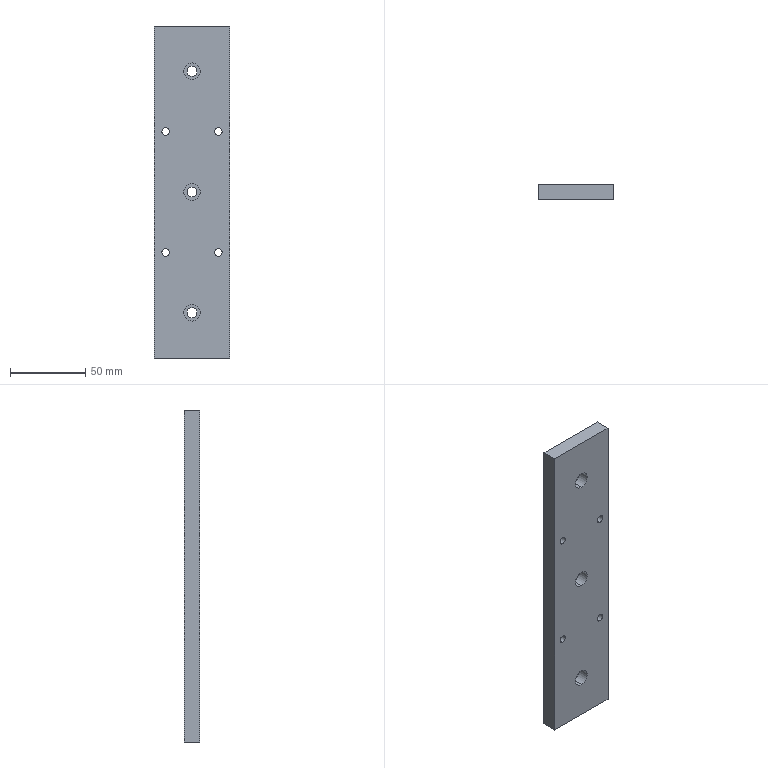Part | SolidWorks | features HoleWzd 2, Extrusion 1 | 1 solid | 29 faces | box 50 x 10 x 220 mm | volume 106947 mm3 | cylinder 20 | plane 9 | commonest cylinder face diameters 5 x8 6.6 x6 11 x6
STEP:
#1=CARTESIAN_POINT('',(-17.5,0.,-37.5));
#2=VERTEX_POINT('',#1);
#3=CARTESIAN_POINT('',(-17.5,0.,-42.5));
#4=VERTEX_POINT('',#3);
#5=CARTESIAN_POINT('',(-17.5,0.,-40.));
#6=DIRECTION('',(0.,-1.,0.));
#7=DIRECTION('',(0.,0.,-1.));
#8=AXIS2_PLACEMENT_3D('',#5,#6,#7);
#9=CIRCLE('',#8,2.5);
#10=EDGE_CURVE('',#2,#4,#9,.T.);
#11=ORIENTED_EDGE('',*,*,#10,.T.);
#12=CARTESIAN_POINT('',(-17.5,10.,-42.5));
#13=VERTEX_POINT('',#12);
#14=CARTESIAN_POINT('',(-17.5,10.,-42.5));
#15=DIRECTION('',(0.,1.,0.));
#16=VECTOR('',#15,1000.);
#17=LINE('',#14,#16);
#18=EDGE_CURVE('',#4,#13,#17,.T.);
#19=ORIENTED_EDGE('',*,*,#18,.T.);
#20=CARTESIAN_POINT('',(-17.5,10.,-37.5));
#21=VERTEX_POINT('',#20);
#22=CARTESIAN_POINT('',(-17.5,10.,-40.));
#23=DIRECTION('',(0.,1.,0.));
#24=DIRECTION('',(0.,0.,1.));
#25=AXIS2_PLACEMENT_3D('',#22,#23,#24);
#26=CIRCLE('',#25,2.5);
#27=EDGE_CURVE('',#13,#21,#26,.T.);
#28=ORIENTED_EDGE('',*,*,#27,.T.);
#29=CARTESIAN_POINT('',(-17.5,10.,-37.5));
#30=DIRECTION('',(0.,1.,0.));
#31=VECTOR('',#30,1000.);
#32=LINE('',#29,#31);
#33=EDGE_CURVE('',#2,#21,#32,.T.);
#34=ORIENTED_EDGE('',*,*,#33,.F.);
#35=EDGE_LOOP('',(#11,#19,#28,#34));
#36=FACE_OUTER_BOUND('',#35,.T.);
#37=CARTESIAN_POINT('',(-17.5,10.,-40.));
#38=DIRECTION('',(0.,1.,0.));
#39=DIRECTION('',(0.,0.,1.));
#40=AXIS2_PLACEMENT_3D('',#37,#38,#39);
#41=CYLINDRICAL_SURFACE('',#40,2.5);
#42=ADVANCED_FACE('',(#36),#41,.F.);
#43=CARTESIAN_POINT('',(-17.5,0.,42.5));
#44=VERTEX_POINT('',#43);
#45=CARTESIAN_POINT('',(-17.5,0.,37.5));
#46=VERTEX_POINT('',#45);
#47=CARTESIAN_POINT('',(-17.5,0.,40.));
#48=DIRECTION('',(0.,-1.,0.));
#49=DIRECTION('',(0.,0.,-1.));
#50=AXIS2_PLACEMENT_3D('',#47,#48,#49);
#51=CIRCLE('',#50,2.5);
#52=EDGE_CURVE('',#44,#46,#51,.T.);
#53=ORIENTED_EDGE('',*,*,#52,.T.);
#54=CARTESIAN_POINT('',(-17.5,10.,37.5));
#55=VERTEX_POINT('',#54);
#56=CARTESIAN_POINT('',(-17.5,10.,37.5));
#57=DIRECTION('',(0.,1.,0.));
#58=VECTOR('',#57,1000.);
#59=LINE('',#56,#58);
#60=EDGE_CURVE('',#46,#55,#59,.T.);
#61=ORIENTED_EDGE('',*,*,#60,.T.);
#62=CARTESIAN_POINT('',(-17.5,10.,42.5));
#63=VERTEX_POINT('',#62);
#64=CARTESIAN_POINT('',(-17.5,10.,40.));
#65=DIRECTION('',(0.,1.,0.));
#66=DIRECTION('',(0.,0.,1.));
#67=AXIS2_PLACEMENT_3D('',#64,#65,#66);
#68=CIRCLE('',#67,2.5);
#69=EDGE_CURVE('',#55,#63,#68,.T.);
#70=ORIENTED_EDGE('',*,*,#69,.T.);
#71=CARTESIAN_POINT('',(-17.5,10.,42.5));
#72=DIRECTION('',(0.,1.,0.));
#73=VECTOR('',#72,1000.);
#74=LINE('',#71,#73);
#75=EDGE_CURVE('',#44,#63,#74,.T.);
#76=ORIENTED_EDGE('',*,*,#75,.F.);
#77=EDGE_LOOP('',(#53,#61,#70,#76));
#78=FACE_OUTER_BOUND('',#77,.T.);
#79=CARTESIAN_POINT('',(-17.5,10.,40.));
#80=DIRECTION('',(0.,1.,0.));
#81=DIRECTION('',(0.,0.,1.));
#82=AXIS2_PLACEMENT_3D('',#79,#80,#81);
#83=CYLINDRICAL_SURFACE('',#82,2.5);
#84=ADVANCED_FACE('',(#78),#83,.F.);
#85=CARTESIAN_POINT('',(17.5,0.,-37.5));
#86=VERTEX_POINT('',#85);
#87=CARTESIAN_POINT('',(17.5,0.,-42.5));
#88=VERTEX_POINT('',#87);
#89=CARTESIAN_POINT('',(17.5,0.,-40.));
#90=DIRECTION('',(0.,-1.,0.));
#91=DIRECTION('',(0.,0.,-1.));
#92=AXIS2_PLACEMENT_3D('',#89,#90,#91);
#93=CIRCLE('',#92,2.5);
#94=EDGE_CURVE('',#86,#88,#93,.T.);
#95=ORIENTED_EDGE('',*,*,#94,.T.);
#96=CARTESIAN_POINT('',(17.5,10.,-42.5));
#97=VERTEX_POINT('',#96);
#98=CARTESIAN_POINT('',(17.5,10.,-42.5));
#99=DIRECTION('',(0.,1.,0.));
#100=VECTOR('',#99,1000.);
#101=LINE('',#98,#100);
#102=EDGE_CURVE('',#88,#97,#101,.T.);
#103=ORIENTED_EDGE('',*,*,#102,.T.);
#104=CARTESIAN_POINT('',(17.5,10.,-37.5));
#105=VERTEX_POINT('',#104);
#106=CARTESIAN_POINT('',(17.5,10.,-40.));
#107=DIRECTION('',(0.,1.,0.));
#108=DIRECTION('',(0.,0.,1.));
#109=AXIS2_PLACEMENT_3D('',#106,#107,#108);
#110=CIRCLE('',#109,2.5);
#111=EDGE_CURVE('',#97,#105,#110,.T.);
#112=ORIENTED_EDGE('',*,*,#111,.T.);
#113=CARTESIAN_POINT('',(17.5,10.,-37.5));
#114=DIRECTION('',(0.,1.,0.));
#115=VECTOR('',#114,1000.);
#116=LINE('',#113,#115);
#117=EDGE_CURVE('',#86,#105,#116,.T.);
#118=ORIENTED_EDGE('',*,*,#117,.F.);
#119=EDGE_LOOP('',(#95,#103,#112,#118));
#120=FACE_OUTER_BOUND('',#119,.T.);
#121=CARTESIAN_POINT('',(17.5,10.,-40.));
#122=DIRECTION('',(0.,1.,0.));
#123=DIRECTION('',(0.,0.,1.));
#124=AXIS2_PLACEMENT_3D('',#121,#122,#123);
#125=CYLINDRICAL_SURFACE('',#124,2.5);
#126=ADVANCED_FACE('',(#120),#125,.F.);
#127=CARTESIAN_POINT('',(17.5,0.,42.5));
#128=VERTEX_POINT('',#127);
#129=CARTESIAN_POINT('',(17.5,0.,37.5));
#130=VERTEX_POINT('',#129);
#131=CARTESIAN_POINT('',(17.5,0.,40.));
#132=DIRECTION('',(0.,-1.,0.));
#133=DIRECTION('',(0.,0.,-1.));
#134=AXIS2_PLACEMENT_3D('',#131,#132,#133);
#135=CIRCLE('',#134,2.5);
#136=EDGE_CURVE('',#128,#130,#135,.T.);
#137=ORIENTED_EDGE('',*,*,#136,.T.);
#138=CARTESIAN_POINT('',(17.5,10.,37.5));
#139=VERTEX_POINT('',#138);
#140=CARTESIAN_POINT('',(17.5,10.,37.5));
#141=DIRECTION('',(0.,1.,0.));
#142=VECTOR('',#141,1000.);
#143=LINE('',#140,#142);
#144=EDGE_CURVE('',#130,#139,#143,.T.);
#145=ORIENTED_EDGE('',*,*,#144,.T.);
#146=CARTESIAN_POINT('',(17.5,10.,42.5));
#147=VERTEX_POINT('',#146);
#148=CARTESIAN_POINT('',(17.5,10.,40.));
#149=DIRECTION('',(0.,1.,0.));
#150=DIRECTION('',(0.,0.,1.));
#151=AXIS2_PLACEMENT_3D('',#148,#149,#150);
#152=CIRCLE('',#151,2.5);
#153=EDGE_CURVE('',#139,#147,#152,.T.);
#154=ORIENTED_EDGE('',*,*,#153,.T.);
#155=CARTESIAN_POINT('',(17.5,10.,42.5));
#156=DIRECTION('',(0.,1.,0.));
#157=VECTOR('',#156,1000.);
#158=LINE('',#155,#157);
#159=EDGE_CURVE('',#128,#147,#158,.T.);
#160=ORIENTED_EDGE('',*,*,#159,.F.);
#161=EDGE_LOOP('',(#137,#145,#154,#160));
#162=FACE_OUTER_BOUND('',#161,.T.);
#163=CARTESIAN_POINT('',(17.5,10.,40.));
#164=DIRECTION('',(0.,1.,0.));
#165=DIRECTION('',(0.,0.,1.));
#166=AXIS2_PLACEMENT_3D('',#163,#164,#165);
#167=CYLINDRICAL_SURFACE('',#166,2.5);
#168=ADVANCED_FACE('',(#162),#167,.F.);
#169=CARTESIAN_POINT('',(0.,6.8,85.5));
#170=VERTEX_POINT('',#169);
#171=CARTESIAN_POINT('',(0.,6.8,74.5));
#172=VERTEX_POINT('',#171);
#173=CARTESIAN_POINT('',(0.,6.8,80.));
#174=DIRECTION('',(0.,-1.,0.));
#175=DIRECTION('',(0.,0.,-1.));
#176=AXIS2_PLACEMENT_3D('',#173,#174,#175);
#177=CIRCLE('',#176,5.5);
#178=EDGE_CURVE('',#170,#172,#177,.T.);
#179=ORIENTED_EDGE('',*,*,#178,.F.);
#180=CARTESIAN_POINT('',(0.,0.,85.5));
#181=VERTEX_POINT('',#180);
#182=CARTESIAN_POINT('',(0.,0.,85.5));
#183=DIRECTION('',(0.,-1.,0.));
#184=VECTOR('',#183,1000.);
#185=LINE('',#182,#184);
#186=EDGE_CURVE('',#170,#181,#185,.T.);
#187=ORIENTED_EDGE('',*,*,#186,.T.);
#188=CARTESIAN_POINT('',(0.,0.,74.5));
#189=VERTEX_POINT('',#188);
#190=CARTESIAN_POINT('',(0.,0.,80.));
#191=DIRECTION('',(0.,-1.,0.));
#192=DIRECTION('',(0.,0.,-1.));
#193=AXIS2_PLACEMENT_3D('',#190,#191,#192);
#194=CIRCLE('',#193,5.5);
#195=EDGE_CURVE('',#181,#189,#194,.T.);
#196=ORIENTED_EDGE('',*,*,#195,.T.);
#197=CARTESIAN_POINT('',(0.,0.,74.5));
#198=DIRECTION('',(0.,-1.,0.));
#199=VECTOR('',#198,1000.);
#200=LINE('',#197,#199);
#201=EDGE_CURVE('',#172,#189,#200,.T.);
#202=ORIENTED_EDGE('',*,*,#201,.F.);
#203=EDGE_LOOP('',(#179,#187,#196,#202));
#204=FACE_OUTER_BOUND('',#203,.T.);
#205=CARTESIAN_POINT('',(0.,0.,80.));
#206=DIRECTION('',(0.,-1.,0.));
#207=DIRECTION('',(0.,0.,-1.));
#208=AXIS2_PLACEMENT_3D('',#205,#206,#207);
#209=CYLINDRICAL_SURFACE('',#208,5.5);
#210=ADVANCED_FACE('',(#204),#209,.F.);
#211=CARTESIAN_POINT('',(0.,10.,83.3));
#212=VERTEX_POINT('',#211);
#213=CARTESIAN_POINT('',(0.,10.,76.7));
#214=VERTEX_POINT('',#213);
#215=CARTESIAN_POINT('',(0.,10.,80.));
#216=DIRECTION('',(0.,-1.,0.));
#217=DIRECTION('',(0.,0.,-1.));
#218=AXIS2_PLACEMENT_3D('',#215,#216,#217);
#219=CIRCLE('',#218,3.3);
#220=EDGE_CURVE('',#212,#214,#219,.T.);
#221=ORIENTED_EDGE('',*,*,#220,.F.);
#222=CARTESIAN_POINT('',(0.,6.8,83.3));
#223=VERTEX_POINT('',#222);
#224=CARTESIAN_POINT('',(0.,0.,83.3));
#225=DIRECTION('',(0.,-1.,0.));
#226=VECTOR('',#225,1000.);
#227=LINE('',#224,#226);
#228=EDGE_CURVE('',#212,#223,#227,.T.);
#229=ORIENTED_EDGE('',*,*,#228,.T.);
#230=CARTESIAN_POINT('',(0.,6.8,76.7));
#231=VERTEX_POINT('',#230);
#232=CARTESIAN_POINT('',(0.,6.8,80.));
#233=DIRECTION('',(0.,-1.,0.));
#234=DIRECTION('',(0.,0.,-1.));
#235=AXIS2_PLACEMENT_3D('',#232,#233,#234);
#236=CIRCLE('',#235,3.3);
#237=EDGE_CURVE('',#223,#231,#236,.T.);
#238=ORIENTED_EDGE('',*,*,#237,.T.);
#239=CARTESIAN_POINT('',(0.,0.,76.7));
#240=DIRECTION('',(0.,-1.,0.));
#241=VECTOR('',#240,1000.);
#242=LINE('',#239,#241);
#243=EDGE_CURVE('',#214,#231,#242,.T.);
#244=ORIENTED_EDGE('',*,*,#243,.F.);
#245=EDGE_LOOP('',(#221,#229,#238,#244));
#246=FACE_OUTER_BOUND('',#245,.T.);
#247=CARTESIAN_POINT('',(0.,0.,80.));
#248=DIRECTION('',(0.,-1.,0.));
#249=DIRECTION('',(0.,0.,-1.));
#250=AXIS2_PLACEMENT_3D('',#247,#248,#249);
#251=CYLINDRICAL_SURFACE('',#250,3.3);
#252=ADVANCED_FACE('',(#246),#251,.F.);
#253=CARTESIAN_POINT('',(0.,6.8,-74.5));
#254=VERTEX_POINT('',#253);
#255=CARTESIAN_POINT('',(0.,6.8,-85.5));
#256=VERTEX_POINT('',#255);
#257=CARTESIAN_POINT('',(0.,6.8,-80.));
#258=DIRECTION('',(0.,-1.,0.));
#259=DIRECTION('',(0.,0.,-1.));
#260=AXIS2_PLACEMENT_3D('',#257,#258,#259);
#261=CIRCLE('',#260,5.5);
#262=EDGE_CURVE('',#254,#256,#261,.T.);
#263=ORIENTED_EDGE('',*,*,#262,.F.);
#264=CARTESIAN_POINT('',(0.,0.,-74.5));
#265=VERTEX_POINT('',#264);
#266=CARTESIAN_POINT('',(0.,0.,-74.5));
#267=DIRECTION('',(0.,-1.,0.));
#268=VECTOR('',#267,1000.);
#269=LINE('',#266,#268);
#270=EDGE_CURVE('',#254,#265,#269,.T.);
#271=ORIENTED_EDGE('',*,*,#270,.T.);
#272=CARTESIAN_POINT('',(0.,0.,-85.5));
#273=VERTEX_POINT('',#272);
#274=CARTESIAN_POINT('',(0.,0.,-80.));
#275=DIRECTION('',(0.,-1.,0.));
#276=DIRECTION('',(0.,0.,-1.));
#277=AXIS2_PLACEMENT_3D('',#274,#275,#276);
#278=CIRCLE('',#277,5.5);
#279=EDGE_CURVE('',#265,#273,#278,.T.);
#280=ORIENTED_EDGE('',*,*,#279,.T.);
#281=CARTESIAN_POINT('',(0.,0.,-85.5));
#282=DIRECTION('',(0.,-1.,0.));
#283=VECTOR('',#282,1000.);
#284=LINE('',#281,#283);
#285=EDGE_CURVE('',#256,#273,#284,.T.);
#286=ORIENTED_EDGE('',*,*,#285,.F.);
#287=EDGE_LOOP('',(#263,#271,#280,#286));
#288=FACE_OUTER_BOUND('',#287,.T.);
#289=CARTESIAN_POINT('',(0.,0.,-80.));
#290=DIRECTION('',(0.,-1.,0.));
#291=DIRECTION('',(0.,0.,-1.));
#292=AXIS2_PLACEMENT_3D('',#289,#290,#291);
#293=CYLINDRICAL_SURFACE('',#292,5.5);
#294=ADVANCED_FACE('',(#288),#293,.F.);
#295=CARTESIAN_POINT('',(0.,10.,-76.7));
#296=VERTEX_POINT('',#295);
#297=CARTESIAN_POINT('',(0.,10.,-83.3));
#298=VERTEX_POINT('',#297);
#299=CARTESIAN_POINT('',(0.,10.,-80.));
#300=DIRECTION('',(0.,-1.,0.));
#301=DIRECTION('',(0.,0.,-1.));
#302=AXIS2_PLACEMENT_3D('',#299,#300,#301);
#303=CIRCLE('',#302,3.3);
#304=EDGE_CURVE('',#296,#298,#303,.T.);
#305=ORIENTED_EDGE('',*,*,#304,.F.);
#306=CARTESIAN_POINT('',(0.,6.8,-76.7));
#307=VERTEX_POINT('',#306);
#308=CARTESIAN_POINT('',(0.,0.,-76.7));
#309=DIRECTION('',(0.,-1.,0.));
#310=VECTOR('',#309,1000.);
#311=LINE('',#308,#310);
#312=EDGE_CURVE('',#296,#307,#311,.T.);
#313=ORIENTED_EDGE('',*,*,#312,.T.);
#314=CARTESIAN_POINT('',(0.,6.8,-83.3));
#315=VERTEX_POINT('',#314);
#316=CARTESIAN_POINT('',(0.,6.8,-80.));
#317=DIRECTION('',(0.,-1.,0.));
#318=DIRECTION('',(0.,0.,-1.));
#319=AXIS2_PLACEMENT_3D('',#316,#317,#318);
#320=CIRCLE('',#319,3.3);
#321=EDGE_CURVE('',#307,#315,#320,.T.);
#322=ORIENTED_EDGE('',*,*,#321,.T.);
#323=CARTESIAN_POINT('',(0.,0.,-83.3));
#324=DIRECTION('',(0.,-1.,0.));
#325=VECTOR('',#324,1000.);
#326=LINE('',#323,#325);
#327=EDGE_CURVE('',#298,#315,#326,.T.);
#328=ORIENTED_EDGE('',*,*,#327,.F.);
#329=EDGE_LOOP('',(#305,#313,#322,#328));
#330=FACE_OUTER_BOUND('',#329,.T.);
#331=CARTESIAN_POINT('',(0.,0.,-80.));
#332=DIRECTION('',(0.,-1.,0.));
#333=DIRECTION('',(0.,0.,-1.));
#334=AXIS2_PLACEMENT_3D('',#331,#332,#333);
#335=CYLINDRICAL_SURFACE('',#334,3.3);
#336=ADVANCED_FACE('',(#330),#335,.F.);
#337=CARTESIAN_POINT('',(0.,6.8,5.5));
#338=VERTEX_POINT('',#337);
#339=CARTESIAN_POINT('',(0.,6.8,-5.5));
#340=VERTEX_POINT('',#339);
#341=CARTESIAN_POINT('',(0.,6.8,0.));
#342=DIRECTION('',(0.,-1.,0.));
#343=DIRECTION('',(0.,0.,-1.));
#344=AXIS2_PLACEMENT_3D('',#341,#342,#343);
#345=CIRCLE('',#344,5.5);
#346=EDGE_CURVE('',#338,#340,#345,.T.);
#347=ORIENTED_EDGE('',*,*,#346,.F.);
#348=CARTESIAN_POINT('',(0.,0.,5.5));
#349=VERTEX_POINT('',#348);
#350=CARTESIAN_POINT('',(0.,0.,5.5));
#351=DIRECTION('',(0.,-1.,0.));
#352=VECTOR('',#351,1000.);
#353=LINE('',#350,#352);
#354=EDGE_CURVE('',#338,#349,#353,.T.);
#355=ORIENTED_EDGE('',*,*,#354,.T.);
#356=CARTESIAN_POINT('',(0.,0.,-5.5));
#357=VERTEX_POINT('',#356);
#358=CARTESIAN_POINT('',(0.,0.,0.));
#359=DIRECTION('',(0.,-1.,0.));
#360=DIRECTION('',(0.,0.,-1.));
#361=AXIS2_PLACEMENT_3D('',#358,#359,#360);
#362=CIRCLE('',#361,5.5);
#363=EDGE_CURVE('',#349,#357,#362,.T.);
#364=ORIENTED_EDGE('',*,*,#363,.T.);
#365=CARTESIAN_POINT('',(0.,0.,-5.5));
#366=DIRECTION('',(0.,-1.,0.));
#367=VECTOR('',#366,1000.);
#368=LINE('',#365,#367);
#369=EDGE_CURVE('',#340,#357,#368,.T.);
#370=ORIENTED_EDGE('',*,*,#369,.F.);
#371=EDGE_LOOP('',(#347,#355,#364,#370));
#372=FACE_OUTER_BOUND('',#371,.T.);
#373=CARTESIAN_POINT('',(0.,0.,0.));
#374=DIRECTION('',(0.,-1.,0.));
#375=DIRECTION('',(0.,0.,-1.));
#376=AXIS2_PLACEMENT_3D('',#373,#374,#375);
#377=CYLINDRICAL_SURFACE('',#376,5.5);
#378=ADVANCED_FACE('',(#372),#377,.F.);
#379=CARTESIAN_POINT('',(0.,10.,3.3));
#380=VERTEX_POINT('',#379);
#381=CARTESIAN_POINT('',(0.,10.,-3.3));
#382=VERTEX_POINT('',#381);
#383=CARTESIAN_POINT('',(0.,10.,0.));
#384=DIRECTION('',(0.,-1.,0.));
#385=DIRECTION('',(0.,0.,-1.));
#386=AXIS2_PLACEMENT_3D('',#383,#384,#385);
#387=CIRCLE('',#386,3.3);
#388=EDGE_CURVE('',#380,#382,#387,.T.);
#389=ORIENTED_EDGE('',*,*,#388,.F.);
#390=CARTESIAN_POINT('',(0.,6.8,3.3));
#391=VERTEX_POINT('',#390);
#392=CARTESIAN_POINT('',(0.,0.,3.3));
#393=DIRECTION('',(0.,-1.,0.));
#394=VECTOR('',#393,1000.);
#395=LINE('',#392,#394);
#396=EDGE_CURVE('',#380,#391,#395,.T.);
#397=ORIENTED_EDGE('',*,*,#396,.T.);
#398=CARTESIAN_POINT('',(0.,6.8,-3.3));
#399=VERTEX_POINT('',#398);
#400=CARTESIAN_POINT('',(0.,6.8,0.));
#401=DIRECTION('',(0.,-1.,0.));
#402=DIRECTION('',(0.,0.,-1.));
#403=AXIS2_PLACEMENT_3D('',#400,#401,#402);
#404=CIRCLE('',#403,3.3);
#405=EDGE_CURVE('',#391,#399,#404,.T.);
#406=ORIENTED_EDGE('',*,*,#405,.T.);
#407=CARTESIAN_POINT('',(0.,0.,-3.3));
#408=DIRECTION('',(0.,-1.,0.));
#409=VECTOR('',#408,1000.);
#410=LINE('',#407,#409);
#411=EDGE_CURVE('',#382,#399,#410,.T.);
#412=ORIENTED_EDGE('',*,*,#411,.F.);
#413=EDGE_LOOP('',(#389,#397,#406,#412));
#414=FACE_OUTER_BOUND('',#413,.T.);
#415=CARTESIAN_POINT('',(0.,0.,0.));
#416=DIRECTION('',(0.,-1.,0.));
#417=DIRECTION('',(0.,0.,-1.));
#418=AXIS2_PLACEMENT_3D('',#415,#416,#417);
#419=CYLINDRICAL_SURFACE('',#418,3.3);
#420=ADVANCED_FACE('',(#414),#419,.F.);
#421=CARTESIAN_POINT('',(25.,0.,110.));
#422=VERTEX_POINT('',#421);
#423=CARTESIAN_POINT('',(25.,0.,-110.));
#424=VERTEX_POINT('',#423);
#425=CARTESIAN_POINT('',(25.,0.,110.));
#426=DIRECTION('',(0.,0.,-1.));
#427=VECTOR('',#426,1000.);
#428=LINE('',#425,#427);
#429=EDGE_CURVE('',#422,#424,#428,.T.);
#430=ORIENTED_EDGE('',*,*,#429,.T.);
#431=CARTESIAN_POINT('',(25.,10.,-110.));
#432=VERTEX_POINT('',#431);
#433=CARTESIAN_POINT('',(25.,10.,-110.));
#434=DIRECTION('',(0.,-1.,0.));
#435=VECTOR('',#434,1000.);
#436=LINE('',#433,#435);
#437=EDGE_CURVE('',#432,#424,#436,.T.);
#438=ORIENTED_EDGE('',*,*,#437,.F.);
#439=CARTESIAN_POINT('',(25.,10.,110.));
#440=VERTEX_POINT('',#439);
#441=CARTESIAN_POINT('',(25.,10.,110.));
#442=DIRECTION('',(0.,0.,-1.));
#443=VECTOR('',#442,1000.);
#444=LINE('',#441,#443);
#445=EDGE_CURVE('',#440,#432,#444,.T.);
#446=ORIENTED_EDGE('',*,*,#445,.F.);
#447=CARTESIAN_POINT('',(25.,10.,110.));
#448=DIRECTION('',(0.,-1.,0.));
#449=VECTOR('',#448,1000.);
#450=LINE('',#447,#449);
#451=EDGE_CURVE('',#440,#422,#450,.T.);
#452=ORIENTED_EDGE('',*,*,#451,.T.);
#453=EDGE_LOOP('',(#430,#438,#446,#452));
#454=FACE_OUTER_BOUND('',#453,.T.);
#455=CARTESIAN_POINT('',(25.,10.,110.));
#456=DIRECTION('',(-1.,0.,0.));
#457=DIRECTION('',(0.,0.,1.));
#458=AXIS2_PLACEMENT_3D('',#455,#456,#457);
#459=PLANE('',#458);
#460=ADVANCED_FACE('',(#454),#459,.F.);
#461=CARTESIAN_POINT('',(-25.,0.,-110.));
#462=VERTEX_POINT('',#461);
#463=CARTESIAN_POINT('',(-25.,0.,-110.));
#464=DIRECTION('',(-1.,0.,0.));
#465=VECTOR('',#464,1000.);
#466=LINE('',#463,#465);
#467=EDGE_CURVE('',#424,#462,#466,.T.);
#468=ORIENTED_EDGE('',*,*,#467,.T.);
#469=CARTESIAN_POINT('',(-25.,10.,-110.));
#470=VERTEX_POINT('',#469);
#471=CARTESIAN_POINT('',(-25.,10.,-110.));
#472=DIRECTION('',(0.,-1.,0.));
#473=VECTOR('',#472,1000.);
#474=LINE('',#471,#473);
#475=EDGE_CURVE('',#470,#462,#474,.T.);
#476=ORIENTED_EDGE('',*,*,#475,.F.);
#477=CARTESIAN_POINT('',(-25.,10.,-110.));
#478=DIRECTION('',(-1.,0.,0.));
#479=VECTOR('',#478,1000.);
#480=LINE('',#477,#479);
#481=EDGE_CURVE('',#432,#470,#480,.T.);
#482=ORIENTED_EDGE('',*,*,#481,.F.);
#483=ORIENTED_EDGE('',*,*,#437,.T.);
#484=EDGE_LOOP('',(#468,#476,#482,#483));
#485=FACE_OUTER_BOUND('',#484,.T.);
#486=CARTESIAN_POINT('',(-25.,10.,-110.));
#487=DIRECTION('',(0.,0.,1.));
#488=DIRECTION('',(1.,0.,0.));
#489=AXIS2_PLACEMENT_3D('',#486,#487,#488);
#490=PLANE('',#489);
#491=ADVANCED_FACE('',(#485),#490,.F.);
#492=CARTESIAN_POINT('',(-25.,0.,110.));
#493=VERTEX_POINT('',#492);
#494=CARTESIAN_POINT('',(-25.,0.,110.));
#495=DIRECTION('',(0.,0.,1.));
#496=VECTOR('',#495,1000.);
#497=LINE('',#494,#496);
#498=EDGE_CURVE('',#462,#493,#497,.T.);
#499=ORIENTED_EDGE('',*,*,#498,.T.);
#500=CARTESIAN_POINT('',(-25.,10.,110.));
#501=VERTEX_POINT('',#500);
#502=CARTESIAN_POINT('',(-25.,10.,110.));
#503=DIRECTION('',(0.,-1.,0.));
#504=VECTOR('',#503,1000.);
#505=LINE('',#502,#504);
#506=EDGE_CURVE('',#501,#493,#505,.T.);
#507=ORIENTED_EDGE('',*,*,#506,.F.);
#508=CARTESIAN_POINT('',(-25.,10.,110.));
#509=DIRECTION('',(0.,0.,1.));
#510=VECTOR('',#509,1000.);
#511=LINE('',#508,#510);
#512=EDGE_CURVE('',#470,#501,#511,.T.);
#513=ORIENTED_EDGE('',*,*,#512,.F.);
#514=ORIENTED_EDGE('',*,*,#475,.T.);
#515=EDGE_LOOP('',(#499,#507,#513,#514));
#516=FACE_OUTER_BOUND('',#515,.T.);
#517=CARTESIAN_POINT('',(-25.,10.,110.));
#518=DIRECTION('',(1.,0.,0.));
#519=DIRECTION('',(0.,0.,-1.));
#520=AXIS2_PLACEMENT_3D('',#517,#518,#519);
#521=PLANE('',#520);
#522=ADVANCED_FACE('',(#516),#521,.F.);
#523=CARTESIAN_POINT('',(-25.,0.,110.));
#524=DIRECTION('',(1.,0.,0.));
#525=VECTOR('',#524,1000.);
#526=LINE('',#523,#525);
#527=EDGE_CURVE('',#493,#422,#526,.T.);
#528=ORIENTED_EDGE('',*,*,#527,.T.);
#529=ORIENTED_EDGE('',*,*,#451,.F.);
#530=CARTESIAN_POINT('',(-25.,10.,110.));
#531=DIRECTION('',(1.,0.,0.));
#532=VECTOR('',#531,1000.);
#533=LINE('',#530,#532);
#534=EDGE_CURVE('',#501,#440,#533,.T.);
#535=ORIENTED_EDGE('',*,*,#534,.F.);
#536=ORIENTED_EDGE('',*,*,#506,.T.);
#537=EDGE_LOOP('',(#528,#529,#535,#536));
#538=FACE_OUTER_BOUND('',#537,.T.);
#539=CARTESIAN_POINT('',(-25.,10.,110.));
#540=DIRECTION('',(0.,0.,-1.));
#541=DIRECTION('',(-1.,0.,0.));
#542=AXIS2_PLACEMENT_3D('',#539,#540,#541);
#543=PLANE('',#542);
#544=ADVANCED_FACE('',(#538),#543,.F.);
#545=CARTESIAN_POINT('',(-17.5,10.,-40.));
#546=DIRECTION('',(0.,1.,0.));
#547=DIRECTION('',(0.,0.,1.));
#548=AXIS2_PLACEMENT_3D('',#545,#546,#547);
#549=CIRCLE('',#548,2.5);
#550=EDGE_CURVE('',#21,#13,#549,.T.);
#551=ORIENTED_EDGE('',*,*,#550,.F.);
#552=ORIENTED_EDGE('',*,*,#27,.F.);
#553=EDGE_LOOP('',(#551,#552));
#554=FACE_BOUND('',#553,.T.);
#555=CARTESIAN_POINT('',(-17.5,10.,40.));
#556=DIRECTION('',(0.,1.,0.));
#557=DIRECTION('',(0.,0.,1.));
#558=AXIS2_PLACEMENT_3D('',#555,#556,#557);
#559=CIRCLE('',#558,2.5);
#560=EDGE_CURVE('',#63,#55,#559,.T.);
#561=ORIENTED_EDGE('',*,*,#560,.F.);
#562=ORIENTED_EDGE('',*,*,#69,.F.);
#563=EDGE_LOOP('',(#561,#562));
#564=FACE_BOUND('',#563,.T.);
#565=CARTESIAN_POINT('',(17.5,10.,-40.));
#566=DIRECTION('',(0.,1.,0.));
#567=DIRECTION('',(0.,0.,1.));
#568=AXIS2_PLACEMENT_3D('',#565,#566,#567);
#569=CIRCLE('',#568,2.5);
#570=EDGE_CURVE('',#105,#97,#569,.T.);
#571=ORIENTED_EDGE('',*,*,#570,.F.);
#572=ORIENTED_EDGE('',*,*,#111,.F.);
#573=EDGE_LOOP('',(#571,#572));
#574=FACE_BOUND('',#573,.T.);
#575=CARTESIAN_POINT('',(17.5,10.,40.));
#576=DIRECTION('',(0.,1.,0.));
#577=DIRECTION('',(0.,0.,1.));
#578=AXIS2_PLACEMENT_3D('',#575,#576,#577);
#579=CIRCLE('',#578,2.5);
#580=EDGE_CURVE('',#147,#139,#579,.T.);
#581=ORIENTED_EDGE('',*,*,#580,.F.);
#582=ORIENTED_EDGE('',*,*,#153,.F.);
#583=EDGE_LOOP('',(#581,#582));
#584=FACE_BOUND('',#583,.T.);
#585=CARTESIAN_POINT('',(0.,10.,80.));
#586=DIRECTION('',(0.,-1.,0.));
#587=DIRECTION('',(0.,0.,-1.));
#588=AXIS2_PLACEMENT_3D('',#585,#586,#587);
#589=CIRCLE('',#588,3.3);
#590=EDGE_CURVE('',#214,#212,#589,.T.);
#591=ORIENTED_EDGE('',*,*,#590,.T.);
#592=ORIENTED_EDGE('',*,*,#220,.T.);
#593=EDGE_LOOP('',(#591,#592));
#594=FACE_BOUND('',#593,.T.);
#595=CARTESIAN_POINT('',(0.,10.,-80.));
#596=DIRECTION('',(0.,-1.,0.));
#597=DIRECTION('',(0.,0.,-1.));
#598=AXIS2_PLACEMENT_3D('',#595,#596,#597);
#599=CIRCLE('',#598,3.3);
#600=EDGE_CURVE('',#298,#296,#599,.T.);
#601=ORIENTED_EDGE('',*,*,#600,.T.);
#602=ORIENTED_EDGE('',*,*,#304,.T.);
#603=EDGE_LOOP('',(#601,#602));
#604=FACE_BOUND('',#603,.T.);
#605=CARTESIAN_POINT('',(0.,10.,0.));
#606=DIRECTION('',(0.,-1.,0.));
#607=DIRECTION('',(0.,0.,-1.));
#608=AXIS2_PLACEMENT_3D('',#605,#606,#607);
#609=CIRCLE('',#608,3.3);
#610=EDGE_CURVE('',#382,#380,#609,.T.);
#611=ORIENTED_EDGE('',*,*,#610,.T.);
#612=ORIENTED_EDGE('',*,*,#388,.T.);
#613=EDGE_LOOP('',(#611,#612));
#614=FACE_BOUND('',#613,.T.);
#615=ORIENTED_EDGE('',*,*,#445,.T.);
#616=ORIENTED_EDGE('',*,*,#481,.T.);
#617=ORIENTED_EDGE('',*,*,#512,.T.);
#618=ORIENTED_EDGE('',*,*,#534,.T.);
#619=EDGE_LOOP('',(#615,#616,#617,#618));
#620=FACE_OUTER_BOUND('',#619,.T.);
#621=CARTESIAN_POINT('',(0.,10.,0.));
#622=DIRECTION('',(0.,-1.,0.));
#623=DIRECTION('',(0.,0.,-1.));
#624=AXIS2_PLACEMENT_3D('',#621,#622,#623);
#625=PLANE('',#624);
#626=ADVANCED_FACE('',(#554,#564,#574,#584,#594,#604,#614,#620),#625,.F.);
#627=ORIENTED_EDGE('',*,*,#10,.F.);
#628=CARTESIAN_POINT('',(-17.5,0.,-40.));
#629=DIRECTION('',(0.,-1.,0.));
#630=DIRECTION('',(0.,0.,-1.));
#631=AXIS2_PLACEMENT_3D('',#628,#629,#630);
#632=CIRCLE('',#631,2.5);
#633=EDGE_CURVE('',#4,#2,#632,.T.);
#634=ORIENTED_EDGE('',*,*,#633,.F.);
#635=EDGE_LOOP('',(#627,#634));
#636=FACE_BOUND('',#635,.T.);
#637=ORIENTED_EDGE('',*,*,#52,.F.);
#638=CARTESIAN_POINT('',(-17.5,0.,40.));
#639=DIRECTION('',(0.,-1.,0.));
#640=DIRECTION('',(0.,0.,-1.));
#641=AXIS2_PLACEMENT_3D('',#638,#639,#640);
#642=CIRCLE('',#641,2.5);
#643=EDGE_CURVE('',#46,#44,#642,.T.);
#644=ORIENTED_EDGE('',*,*,#643,.F.);
#645=EDGE_LOOP('',(#637,#644));
#646=FACE_BOUND('',#645,.T.);
#647=ORIENTED_EDGE('',*,*,#94,.F.);
#648=CARTESIAN_POINT('',(17.5,0.,-40.));
#649=DIRECTION('',(0.,-1.,0.));
#650=DIRECTION('',(0.,0.,-1.));
#651=AXIS2_PLACEMENT_3D('',#648,#649,#650);
#652=CIRCLE('',#651,2.5);
#653=EDGE_CURVE('',#88,#86,#652,.T.);
#654=ORIENTED_EDGE('',*,*,#653,.F.);
#655=EDGE_LOOP('',(#647,#654));
#656=FACE_BOUND('',#655,.T.);
#657=ORIENTED_EDGE('',*,*,#136,.F.);
#658=CARTESIAN_POINT('',(17.5,0.,40.));
#659=DIRECTION('',(0.,-1.,0.));
#660=DIRECTION('',(0.,0.,-1.));
#661=AXIS2_PLACEMENT_3D('',#658,#659,#660);
#662=CIRCLE('',#661,2.5);
#663=EDGE_CURVE('',#130,#128,#662,.T.);
#664=ORIENTED_EDGE('',*,*,#663,.F.);
#665=EDGE_LOOP('',(#657,#664));
#666=FACE_BOUND('',#665,.T.);
#667=CARTESIAN_POINT('',(0.,0.,80.));
#668=DIRECTION('',(0.,-1.,0.));
#669=DIRECTION('',(0.,0.,-1.));
#670=AXIS2_PLACEMENT_3D('',#667,#668,#669);
#671=CIRCLE('',#670,5.5);
#672=EDGE_CURVE('',#189,#181,#671,.T.);
#673=ORIENTED_EDGE('',*,*,#672,.F.);
#674=ORIENTED_EDGE('',*,*,#195,.F.);
#675=EDGE_LOOP('',(#673,#674));
#676=FACE_BOUND('',#675,.T.);
#677=CARTESIAN_POINT('',(0.,0.,-80.));
#678=DIRECTION('',(0.,-1.,0.));
#679=DIRECTION('',(0.,0.,-1.));
#680=AXIS2_PLACEMENT_3D('',#677,#678,#679);
#681=CIRCLE('',#680,5.5);
#682=EDGE_CURVE('',#273,#265,#681,.T.);
#683=ORIENTED_EDGE('',*,*,#682,.F.);
#684=ORIENTED_EDGE('',*,*,#279,.F.);
#685=EDGE_LOOP('',(#683,#684));
#686=FACE_BOUND('',#685,.T.);
#687=CARTESIAN_POINT('',(0.,0.,0.));
#688=DIRECTION('',(0.,-1.,0.));
#689=DIRECTION('',(0.,0.,-1.));
#690=AXIS2_PLACEMENT_3D('',#687,#688,#689);
#691=CIRCLE('',#690,5.5);
#692=EDGE_CURVE('',#357,#349,#691,.T.);
#693=ORIENTED_EDGE('',*,*,#692,.F.);
#694=ORIENTED_EDGE('',*,*,#363,.F.);
#695=EDGE_LOOP('',(#693,#694));
#696=FACE_BOUND('',#695,.T.);
#697=ORIENTED_EDGE('',*,*,#429,.F.);
#698=ORIENTED_EDGE('',*,*,#527,.F.);
#699=ORIENTED_EDGE('',*,*,#498,.F.);
#700=ORIENTED_EDGE('',*,*,#467,.F.);
#701=EDGE_LOOP('',(#697,#698,#699,#700));
#702=FACE_OUTER_BOUND('',#701,.T.);
#703=CARTESIAN_POINT('',(0.,0.,0.));
#704=DIRECTION('',(0.,-1.,0.));
#705=DIRECTION('',(0.,0.,-1.));
#706=AXIS2_PLACEMENT_3D('',#703,#704,#705);
#707=PLANE('',#706);
#708=ADVANCED_FACE('',(#636,#646,#656,#666,#676,#686,#696,#702),#707,.T.);
#709=ORIENTED_EDGE('',*,*,#396,.F.);
#710=ORIENTED_EDGE('',*,*,#610,.F.);
#711=ORIENTED_EDGE('',*,*,#411,.T.);
#712=CARTESIAN_POINT('',(0.,6.8,0.));
#713=DIRECTION('',(0.,-1.,0.));
#714=DIRECTION('',(0.,0.,-1.));
#715=AXIS2_PLACEMENT_3D('',#712,#713,#714);
#716=CIRCLE('',#715,3.3);
#717=EDGE_CURVE('',#399,#391,#716,.T.);
#718=ORIENTED_EDGE('',*,*,#717,.T.);
#719=EDGE_LOOP('',(#709,#710,#711,#718));
#720=FACE_OUTER_BOUND('',#719,.T.);
#721=CARTESIAN_POINT('',(0.,0.,0.));
#722=DIRECTION('',(0.,-1.,0.));
#723=DIRECTION('',(0.,0.,-1.));
#724=AXIS2_PLACEMENT_3D('',#721,#722,#723);
#725=CYLINDRICAL_SURFACE('',#724,3.3);
#726=ADVANCED_FACE('',(#720),#725,.F.);
#727=ORIENTED_EDGE('',*,*,#717,.F.);
#728=ORIENTED_EDGE('',*,*,#405,.F.);
#729=EDGE_LOOP('',(#727,#728));
#730=FACE_BOUND('',#729,.T.);
#731=CARTESIAN_POINT('',(0.,6.8,0.));
#732=DIRECTION('',(0.,-1.,0.));
#733=DIRECTION('',(0.,0.,-1.));
#734=AXIS2_PLACEMENT_3D('',#731,#732,#733);
#735=CIRCLE('',#734,5.5);
#736=EDGE_CURVE('',#340,#338,#735,.T.);
#737=ORIENTED_EDGE('',*,*,#736,.T.);
#738=ORIENTED_EDGE('',*,*,#346,.T.);
#739=EDGE_LOOP('',(#737,#738));
#740=FACE_OUTER_BOUND('',#739,.T.);
#741=CARTESIAN_POINT('',(3.3,6.8,0.));
#742=DIRECTION('',(0.,1.,0.));
#743=DIRECTION('',(0.,0.,1.));
#744=AXIS2_PLACEMENT_3D('',#741,#742,#743);
#745=PLANE('',#744);
#746=ADVANCED_FACE('',(#730,#740),#745,.F.);
#747=ORIENTED_EDGE('',*,*,#354,.F.);
#748=ORIENTED_EDGE('',*,*,#736,.F.);
#749=ORIENTED_EDGE('',*,*,#369,.T.);
#750=ORIENTED_EDGE('',*,*,#692,.T.);
#751=EDGE_LOOP('',(#747,#748,#749,#750));
#752=FACE_OUTER_BOUND('',#751,.T.);
#753=CARTESIAN_POINT('',(0.,0.,0.));
#754=DIRECTION('',(0.,-1.,0.));
#755=DIRECTION('',(0.,0.,-1.));
#756=AXIS2_PLACEMENT_3D('',#753,#754,#755);
#757=CYLINDRICAL_SURFACE('',#756,5.5);
#758=ADVANCED_FACE('',(#752),#757,.F.);
#759=ORIENTED_EDGE('',*,*,#312,.F.);
#760=ORIENTED_EDGE('',*,*,#600,.F.);
#761=ORIENTED_EDGE('',*,*,#327,.T.);
#762=CARTESIAN_POINT('',(0.,6.8,-80.));
#763=DIRECTION('',(0.,-1.,0.));
#764=DIRECTION('',(0.,0.,-1.));
#765=AXIS2_PLACEMENT_3D('',#762,#763,#764);
#766=CIRCLE('',#765,3.3);
#767=EDGE_CURVE('',#315,#307,#766,.T.);
#768=ORIENTED_EDGE('',*,*,#767,.T.);
#769=EDGE_LOOP('',(#759,#760,#761,#768));
#770=FACE_OUTER_BOUND('',#769,.T.);
#771=CARTESIAN_POINT('',(0.,0.,-80.));
#772=DIRECTION('',(0.,-1.,0.));
#773=DIRECTION('',(0.,0.,-1.));
#774=AXIS2_PLACEMENT_3D('',#771,#772,#773);
#775=CYLINDRICAL_SURFACE('',#774,3.3);
#776=ADVANCED_FACE('',(#770),#775,.F.);
#777=ORIENTED_EDGE('',*,*,#767,.F.);
#778=ORIENTED_EDGE('',*,*,#321,.F.);
#779=EDGE_LOOP('',(#777,#778));
#780=FACE_BOUND('',#779,.T.);
#781=CARTESIAN_POINT('',(0.,6.8,-80.));
#782=DIRECTION('',(0.,-1.,0.));
#783=DIRECTION('',(0.,0.,-1.));
#784=AXIS2_PLACEMENT_3D('',#781,#782,#783);
#785=CIRCLE('',#784,5.5);
#786=EDGE_CURVE('',#256,#254,#785,.T.);
#787=ORIENTED_EDGE('',*,*,#786,.T.);
#788=ORIENTED_EDGE('',*,*,#262,.T.);
#789=EDGE_LOOP('',(#787,#788));
#790=FACE_OUTER_BOUND('',#789,.T.);
#791=CARTESIAN_POINT('',(3.3,6.8,-80.));
#792=DIRECTION('',(0.,1.,0.));
#793=DIRECTION('',(0.,0.,1.));
#794=AXIS2_PLACEMENT_3D('',#791,#792,#793);
#795=PLANE('',#794);
#796=ADVANCED_FACE('',(#780,#790),#795,.F.);
#797=ORIENTED_EDGE('',*,*,#270,.F.);
#798=ORIENTED_EDGE('',*,*,#786,.F.);
#799=ORIENTED_EDGE('',*,*,#285,.T.);
#800=ORIENTED_EDGE('',*,*,#682,.T.);
#801=EDGE_LOOP('',(#797,#798,#799,#800));
#802=FACE_OUTER_BOUND('',#801,.T.);
#803=CARTESIAN_POINT('',(0.,0.,-80.));
#804=DIRECTION('',(0.,-1.,0.));
#805=DIRECTION('',(0.,0.,-1.));
#806=AXIS2_PLACEMENT_3D('',#803,#804,#805);
#807=CYLINDRICAL_SURFACE('',#806,5.5);
#808=ADVANCED_FACE('',(#802),#807,.F.);
#809=ORIENTED_EDGE('',*,*,#228,.F.);
#810=ORIENTED_EDGE('',*,*,#590,.F.);
#811=ORIENTED_EDGE('',*,*,#243,.T.);
#812=CARTESIAN_POINT('',(0.,6.8,80.));
#813=DIRECTION('',(0.,-1.,0.));
#814=DIRECTION('',(0.,0.,-1.));
#815=AXIS2_PLACEMENT_3D('',#812,#813,#814);
#816=CIRCLE('',#815,3.3);
#817=EDGE_CURVE('',#231,#223,#816,.T.);
#818=ORIENTED_EDGE('',*,*,#817,.T.);
#819=EDGE_LOOP('',(#809,#810,#811,#818));
#820=FACE_OUTER_BOUND('',#819,.T.);
#821=CARTESIAN_POINT('',(0.,0.,80.));
#822=DIRECTION('',(0.,-1.,0.));
#823=DIRECTION('',(0.,0.,-1.));
#824=AXIS2_PLACEMENT_3D('',#821,#822,#823);
#825=CYLINDRICAL_SURFACE('',#824,3.3);
#826=ADVANCED_FACE('',(#820),#825,.F.);
#827=ORIENTED_EDGE('',*,*,#817,.F.);
#828=ORIENTED_EDGE('',*,*,#237,.F.);
#829=EDGE_LOOP('',(#827,#828));
#830=FACE_BOUND('',#829,.T.);
#831=CARTESIAN_POINT('',(0.,6.8,80.));
#832=DIRECTION('',(0.,-1.,0.));
#833=DIRECTION('',(0.,0.,-1.));
#834=AXIS2_PLACEMENT_3D('',#831,#832,#833);
#835=CIRCLE('',#834,5.5);
#836=EDGE_CURVE('',#172,#170,#835,.T.);
#837=ORIENTED_EDGE('',*,*,#836,.T.);
#838=ORIENTED_EDGE('',*,*,#178,.T.);
#839=EDGE_LOOP('',(#837,#838));
#840=FACE_OUTER_BOUND('',#839,.T.);
#841=CARTESIAN_POINT('',(3.3,6.8,80.));
#842=DIRECTION('',(0.,1.,0.));
#843=DIRECTION('',(0.,0.,1.));
#844=AXIS2_PLACEMENT_3D('',#841,#842,#843);
#845=PLANE('',#844);
#846=ADVANCED_FACE('',(#830,#840),#845,.F.);
#847=ORIENTED_EDGE('',*,*,#186,.F.);
#848=ORIENTED_EDGE('',*,*,#836,.F.);
#849=ORIENTED_EDGE('',*,*,#201,.T.);
#850=ORIENTED_EDGE('',*,*,#672,.T.);
#851=EDGE_LOOP('',(#847,#848,#849,#850));
#852=FACE_OUTER_BOUND('',#851,.T.);
#853=CARTESIAN_POINT('',(0.,0.,80.));
#854=DIRECTION('',(0.,-1.,0.));
#855=DIRECTION('',(0.,0.,-1.));
#856=AXIS2_PLACEMENT_3D('',#853,#854,#855);
#857=CYLINDRICAL_SURFACE('',#856,5.5);
#858=ADVANCED_FACE('',(#852),#857,.F.);
#859=ORIENTED_EDGE('',*,*,#144,.F.);
#860=ORIENTED_EDGE('',*,*,#663,.T.);
#861=ORIENTED_EDGE('',*,*,#159,.T.);
#862=ORIENTED_EDGE('',*,*,#580,.T.);
#863=EDGE_LOOP('',(#859,#860,#861,#862));
#864=FACE_OUTER_BOUND('',#863,.T.);
#865=CARTESIAN_POINT('',(17.5,10.,40.));
#866=DIRECTION('',(0.,1.,0.));
#867=DIRECTION('',(0.,0.,1.));
#868=AXIS2_PLACEMENT_3D('',#865,#866,#867);
#869=CYLINDRICAL_SURFACE('',#868,2.5);
#870=ADVANCED_FACE('',(#864),#869,.F.);
#871=ORIENTED_EDGE('',*,*,#102,.F.);
#872=ORIENTED_EDGE('',*,*,#653,.T.);
#873=ORIENTED_EDGE('',*,*,#117,.T.);
#874=ORIENTED_EDGE('',*,*,#570,.T.);
#875=EDGE_LOOP('',(#871,#872,#873,#874));
#876=FACE_OUTER_BOUND('',#875,.T.);
#877=CARTESIAN_POINT('',(17.5,10.,-40.));
#878=DIRECTION('',(0.,1.,0.));
#879=DIRECTION('',(0.,0.,1.));
#880=AXIS2_PLACEMENT_3D('',#877,#878,#879);
#881=CYLINDRICAL_SURFACE('',#880,2.5);
#882=ADVANCED_FACE('',(#876),#881,.F.);
#883=ORIENTED_EDGE('',*,*,#60,.F.);
#884=ORIENTED_EDGE('',*,*,#643,.T.);
#885=ORIENTED_EDGE('',*,*,#75,.T.);
#886=ORIENTED_EDGE('',*,*,#560,.T.);
#887=EDGE_LOOP('',(#883,#884,#885,#886));
#888=FACE_OUTER_BOUND('',#887,.T.);
#889=CARTESIAN_POINT('',(-17.5,10.,40.));
#890=DIRECTION('',(0.,1.,0.));
#891=DIRECTION('',(0.,0.,1.));
#892=AXIS2_PLACEMENT_3D('',#889,#890,#891);
#893=CYLINDRICAL_SURFACE('',#892,2.5);
#894=ADVANCED_FACE('',(#888),#893,.F.);
#895=ORIENTED_EDGE('',*,*,#18,.F.);
#896=ORIENTED_EDGE('',*,*,#633,.T.);
#897=ORIENTED_EDGE('',*,*,#33,.T.);
#898=ORIENTED_EDGE('',*,*,#550,.T.);
#899=EDGE_LOOP('',(#895,#896,#897,#898));
#900=FACE_OUTER_BOUND('',#899,.T.);
#901=CARTESIAN_POINT('',(-17.5,10.,-40.));
#902=DIRECTION('',(0.,1.,0.));
#903=DIRECTION('',(0.,0.,1.));
#904=AXIS2_PLACEMENT_3D('',#901,#902,#903);
#905=CYLINDRICAL_SURFACE('',#904,2.5);
#906=ADVANCED_FACE('',(#900),#905,.F.);
#907=CLOSED_SHELL('',(#42,#84,#126,#168,#210,#252,#294,#336,#378,#420,#460,#491,#522,#544,#626,#708,#726,#746,#758,#776,#796,#808,#826,#846,#858,#870,#882,#894,#906));
#908=MANIFOLD_SOLID_BREP('',#907);
#909=CARTESIAN_POINT('',(0.,0.,0.));
#910=DIRECTION('',(0.,0.,1.));
#911=DIRECTION('',(1.,0.,0.));
#912=AXIS2_PLACEMENT_3D('',#909,#910,#911);
#913=(LENGTH_UNIT()NAMED_UNIT(*)SI_UNIT(.MILLI.,.METRE.));
#914=UNCERTAINTY_MEASURE_WITH_UNIT(LENGTH_MEASURE(0.00001),#913,'','');
#915=(NAMED_UNIT(*)PLANE_ANGLE_UNIT()SI_UNIT($,.RADIAN.));
#916=(NAMED_UNIT(*)SI_UNIT($,.STERADIAN.)SOLID_ANGLE_UNIT());
#917=(GEOMETRIC_REPRESENTATION_CONTEXT(3)GLOBAL_UNCERTAINTY_ASSIGNED_CONTEXT((#914))GLOBAL_UNIT_ASSIGNED_CONTEXT((#913,#915,#916))REPRESENTATION_CONTEXT('',''));
#918=ADVANCED_BREP_SHAPE_REPRESENTATION('',(#908,#912),#917);